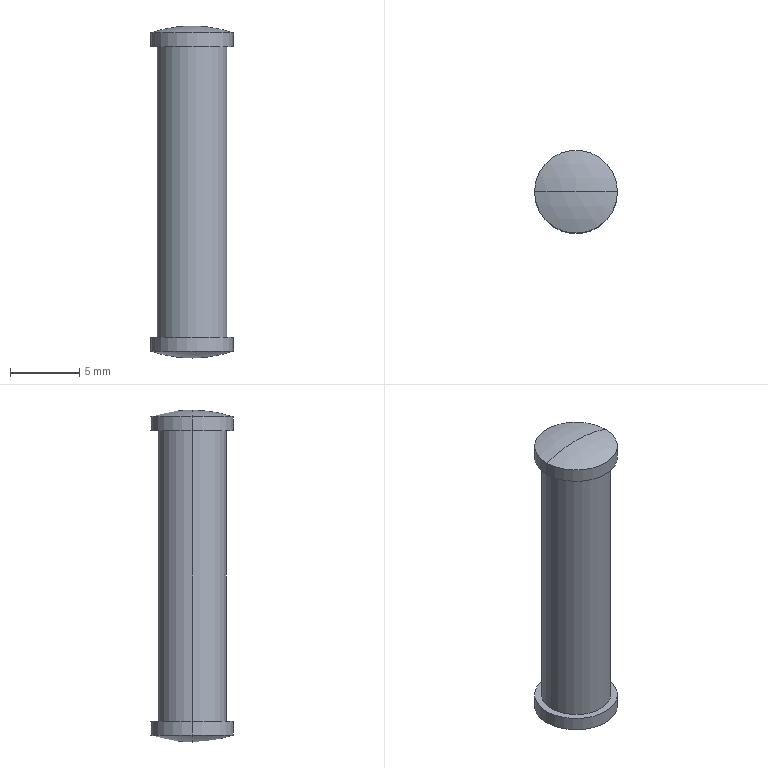Part | SolidWorks | features Dome 2, ICE 2, Extrusion 1 | 1 solid | 12 faces | box 6 x 6 x 24 mm | volume 483.151 mm3 | cylinder 6 | sphere 4 | plane 2 | commonest cylinder face diameters 6 x4 5 x2
STEP:
#1=CARTESIAN_POINT('',(3.,0.,11.5));
#2=VERTEX_POINT('',#1);
#3=CARTESIAN_POINT('',(-3.,0.,11.5));
#4=VERTEX_POINT('',#3);
#5=CARTESIAN_POINT('',(0.,0.,11.5));
#6=DIRECTION('',(0.,0.,1.));
#7=DIRECTION('',(1.,0.,0.));
#8=AXIS2_PLACEMENT_3D('',#5,#6,#7);
#9=CIRCLE('',#8,3.);
#10=EDGE_CURVE('',#2,#4,#9,.T.);
#11=ORIENTED_EDGE('',*,*,#10,.T.);
#12=CARTESIAN_POINT('',(0.,0.,12.));
#13=VERTEX_POINT('',#12);
#14=CARTESIAN_POINT('',(0.,0.,2.75));
#15=DIRECTION('',(0.,1.,0.));
#16=DIRECTION('',(-1.,0.,0.));
#17=AXIS2_PLACEMENT_3D('',#14,#15,#16);
#18=CIRCLE('',#17,9.25);
#19=EDGE_CURVE('',#4,#13,#18,.T.);
#20=ORIENTED_EDGE('',*,*,#19,.T.);
#21=CARTESIAN_POINT('',(0.,0.,2.75));
#22=DIRECTION('',(0.,-1.,0.));
#23=DIRECTION('',(0.,0.,-1.));
#24=AXIS2_PLACEMENT_3D('',#21,#22,#23);
#25=CIRCLE('',#24,9.25);
#26=EDGE_CURVE('',#2,#13,#25,.T.);
#27=ORIENTED_EDGE('',*,*,#26,.F.);
#28=EDGE_LOOP('',(#11,#20,#27));
#29=FACE_OUTER_BOUND('',#28,.T.);
#30=CARTESIAN_POINT('',(0.,0.,2.75));
#31=DIRECTION('',(0.,1.,0.));
#32=DIRECTION('',(1.,0.,0.));
#33=AXIS2_PLACEMENT_3D('',#30,#31,#32);
#34=SPHERICAL_SURFACE('',#33,9.25);
#35=ADVANCED_FACE('',(#29),#34,.T.);
#36=ORIENTED_EDGE('',*,*,#10,.F.);
#37=CARTESIAN_POINT('',(3.,0.,10.5));
#38=VERTEX_POINT('',#37);
#39=CARTESIAN_POINT('',(3.,0.,11.5));
#40=DIRECTION('',(0.,0.,-1.));
#41=VECTOR('',#40,1000.);
#42=LINE('',#39,#41);
#43=EDGE_CURVE('',#2,#38,#42,.T.);
#44=ORIENTED_EDGE('',*,*,#43,.T.);
#45=CARTESIAN_POINT('',(-3.,0.,10.5));
#46=VERTEX_POINT('',#45);
#47=CARTESIAN_POINT('',(0.,0.,10.5));
#48=DIRECTION('',(0.,0.,1.));
#49=DIRECTION('',(1.,0.,0.));
#50=AXIS2_PLACEMENT_3D('',#47,#48,#49);
#51=CIRCLE('',#50,3.);
#52=EDGE_CURVE('',#38,#46,#51,.T.);
#53=ORIENTED_EDGE('',*,*,#52,.T.);
#54=CARTESIAN_POINT('',(-3.,0.,11.5));
#55=DIRECTION('',(0.,0.,-1.));
#56=VECTOR('',#55,1000.);
#57=LINE('',#54,#56);
#58=EDGE_CURVE('',#4,#46,#57,.T.);
#59=ORIENTED_EDGE('',*,*,#58,.F.);
#60=EDGE_LOOP('',(#36,#44,#53,#59));
#61=FACE_OUTER_BOUND('',#60,.T.);
#62=CARTESIAN_POINT('',(0.,0.,11.5));
#63=DIRECTION('',(0.,0.,-1.));
#64=DIRECTION('',(-1.,0.,0.));
#65=AXIS2_PLACEMENT_3D('',#62,#63,#64);
#66=CYLINDRICAL_SURFACE('',#65,3.);
#67=ADVANCED_FACE('',(#61),#66,.T.);
#68=CARTESIAN_POINT('',(0.,0.,-12.));
#69=VERTEX_POINT('',#68);
#70=CARTESIAN_POINT('',(3.,0.,-11.5));
#71=VERTEX_POINT('',#70);
#72=CARTESIAN_POINT('',(0.,0.,-2.75));
#73=DIRECTION('',(0.,-1.,0.));
#74=DIRECTION('',(0.,0.,-1.));
#75=AXIS2_PLACEMENT_3D('',#72,#73,#74);
#76=CIRCLE('',#75,9.25);
#77=EDGE_CURVE('',#69,#71,#76,.T.);
#78=ORIENTED_EDGE('',*,*,#77,.F.);
#79=CARTESIAN_POINT('',(-3.,0.,-11.5));
#80=VERTEX_POINT('',#79);
#81=CARTESIAN_POINT('',(0.,0.,-2.75));
#82=DIRECTION('',(0.,1.,0.));
#83=DIRECTION('',(-1.,0.,0.));
#84=AXIS2_PLACEMENT_3D('',#81,#82,#83);
#85=CIRCLE('',#84,9.25);
#86=EDGE_CURVE('',#69,#80,#85,.T.);
#87=ORIENTED_EDGE('',*,*,#86,.T.);
#88=CARTESIAN_POINT('',(0.,0.,-11.5));
#89=DIRECTION('',(0.,0.,-1.));
#90=DIRECTION('',(-1.,0.,0.));
#91=AXIS2_PLACEMENT_3D('',#88,#89,#90);
#92=CIRCLE('',#91,3.);
#93=EDGE_CURVE('',#80,#71,#92,.T.);
#94=ORIENTED_EDGE('',*,*,#93,.T.);
#95=EDGE_LOOP('',(#78,#87,#94));
#96=FACE_OUTER_BOUND('',#95,.T.);
#97=CARTESIAN_POINT('',(0.,0.,-2.75));
#98=DIRECTION('',(0.,1.,0.));
#99=DIRECTION('',(1.,0.,0.));
#100=AXIS2_PLACEMENT_3D('',#97,#98,#99);
#101=SPHERICAL_SURFACE('',#100,9.25);
#102=ADVANCED_FACE('',(#96),#101,.T.);
#103=ORIENTED_EDGE('',*,*,#93,.F.);
#104=CARTESIAN_POINT('',(-3.,0.,-10.5));
#105=VERTEX_POINT('',#104);
#106=CARTESIAN_POINT('',(-3.,0.,-11.5));
#107=DIRECTION('',(0.,0.,1.));
#108=VECTOR('',#107,1000.);
#109=LINE('',#106,#108);
#110=EDGE_CURVE('',#80,#105,#109,.T.);
#111=ORIENTED_EDGE('',*,*,#110,.T.);
#112=CARTESIAN_POINT('',(3.,0.,-10.5));
#113=VERTEX_POINT('',#112);
#114=CARTESIAN_POINT('',(0.,0.,-10.5));
#115=DIRECTION('',(0.,0.,-1.));
#116=DIRECTION('',(-1.,0.,0.));
#117=AXIS2_PLACEMENT_3D('',#114,#115,#116);
#118=CIRCLE('',#117,3.);
#119=EDGE_CURVE('',#105,#113,#118,.T.);
#120=ORIENTED_EDGE('',*,*,#119,.T.);
#121=CARTESIAN_POINT('',(3.,0.,-11.5));
#122=DIRECTION('',(0.,0.,1.));
#123=VECTOR('',#122,1000.);
#124=LINE('',#121,#123);
#125=EDGE_CURVE('',#71,#113,#124,.T.);
#126=ORIENTED_EDGE('',*,*,#125,.F.);
#127=EDGE_LOOP('',(#103,#111,#120,#126));
#128=FACE_OUTER_BOUND('',#127,.T.);
#129=CARTESIAN_POINT('',(0.,0.,-11.5));
#130=DIRECTION('',(0.,0.,1.));
#131=DIRECTION('',(1.,0.,0.));
#132=AXIS2_PLACEMENT_3D('',#129,#130,#131);
#133=CYLINDRICAL_SURFACE('',#132,3.);
#134=ADVANCED_FACE('',(#128),#133,.T.);
#135=CARTESIAN_POINT('',(2.5,0.,10.5));
#136=VERTEX_POINT('',#135);
#137=CARTESIAN_POINT('',(-2.5,0.,10.5));
#138=VERTEX_POINT('',#137);
#139=CARTESIAN_POINT('',(0.,0.,10.5));
#140=DIRECTION('',(0.,0.,1.));
#141=DIRECTION('',(1.,0.,0.));
#142=AXIS2_PLACEMENT_3D('',#139,#140,#141);
#143=CIRCLE('',#142,2.5);
#144=EDGE_CURVE('',#136,#138,#143,.T.);
#145=ORIENTED_EDGE('',*,*,#144,.F.);
#146=CARTESIAN_POINT('',(2.5,0.,-10.5));
#147=VERTEX_POINT('',#146);
#148=CARTESIAN_POINT('',(2.5,0.,10.5));
#149=DIRECTION('',(0.,0.,-1.));
#150=VECTOR('',#149,1000.);
#151=LINE('',#148,#150);
#152=EDGE_CURVE('',#136,#147,#151,.T.);
#153=ORIENTED_EDGE('',*,*,#152,.T.);
#154=CARTESIAN_POINT('',(-2.5,0.,-10.5));
#155=VERTEX_POINT('',#154);
#156=CARTESIAN_POINT('',(0.,0.,-10.5));
#157=DIRECTION('',(0.,0.,-1.));
#158=DIRECTION('',(-1.,0.,0.));
#159=AXIS2_PLACEMENT_3D('',#156,#157,#158);
#160=CIRCLE('',#159,2.5);
#161=EDGE_CURVE('',#155,#147,#160,.T.);
#162=ORIENTED_EDGE('',*,*,#161,.F.);
#163=CARTESIAN_POINT('',(-2.5,0.,10.5));
#164=DIRECTION('',(0.,0.,-1.));
#165=VECTOR('',#164,1000.);
#166=LINE('',#163,#165);
#167=EDGE_CURVE('',#138,#155,#166,.T.);
#168=ORIENTED_EDGE('',*,*,#167,.F.);
#169=EDGE_LOOP('',(#145,#153,#162,#168));
#170=FACE_OUTER_BOUND('',#169,.T.);
#171=CARTESIAN_POINT('',(0.,0.,10.5));
#172=DIRECTION('',(0.,0.,-1.));
#173=DIRECTION('',(-1.,0.,0.));
#174=AXIS2_PLACEMENT_3D('',#171,#172,#173);
#175=CYLINDRICAL_SURFACE('',#174,2.5);
#176=ADVANCED_FACE('',(#170),#175,.T.);
#177=ORIENTED_EDGE('',*,*,#152,.F.);
#178=CARTESIAN_POINT('',(0.,0.,10.5));
#179=DIRECTION('',(0.,0.,1.));
#180=DIRECTION('',(1.,0.,0.));
#181=AXIS2_PLACEMENT_3D('',#178,#179,#180);
#182=CIRCLE('',#181,2.5);
#183=EDGE_CURVE('',#138,#136,#182,.T.);
#184=ORIENTED_EDGE('',*,*,#183,.F.);
#185=ORIENTED_EDGE('',*,*,#167,.T.);
#186=CARTESIAN_POINT('',(0.,0.,-10.5));
#187=DIRECTION('',(0.,0.,-1.));
#188=DIRECTION('',(-1.,0.,0.));
#189=AXIS2_PLACEMENT_3D('',#186,#187,#188);
#190=CIRCLE('',#189,2.5);
#191=EDGE_CURVE('',#147,#155,#190,.T.);
#192=ORIENTED_EDGE('',*,*,#191,.F.);
#193=EDGE_LOOP('',(#177,#184,#185,#192));
#194=FACE_OUTER_BOUND('',#193,.T.);
#195=CARTESIAN_POINT('',(0.,0.,10.5));
#196=DIRECTION('',(0.,0.,-1.));
#197=DIRECTION('',(-1.,0.,0.));
#198=AXIS2_PLACEMENT_3D('',#195,#196,#197);
#199=CYLINDRICAL_SURFACE('',#198,2.5);
#200=ADVANCED_FACE('',(#194),#199,.T.);
#201=CARTESIAN_POINT('',(0.,0.,-10.5));
#202=DIRECTION('',(0.,0.,-1.));
#203=DIRECTION('',(-1.,0.,0.));
#204=AXIS2_PLACEMENT_3D('',#201,#202,#203);
#205=CIRCLE('',#204,3.);
#206=EDGE_CURVE('',#113,#105,#205,.T.);
#207=ORIENTED_EDGE('',*,*,#206,.F.);
#208=ORIENTED_EDGE('',*,*,#119,.F.);
#209=EDGE_LOOP('',(#207,#208));
#210=FACE_OUTER_BOUND('',#209,.T.);
#211=ORIENTED_EDGE('',*,*,#161,.T.);
#212=ORIENTED_EDGE('',*,*,#191,.T.);
#213=EDGE_LOOP('',(#211,#212));
#214=FACE_BOUND('',#213,.T.);
#215=CARTESIAN_POINT('',(0.,0.,-10.5));
#216=DIRECTION('',(0.,0.,-1.));
#217=DIRECTION('',(-1.,0.,0.));
#218=AXIS2_PLACEMENT_3D('',#215,#216,#217);
#219=PLANE('',#218);
#220=ADVANCED_FACE('',(#210,#214),#219,.F.);
#221=ORIENTED_EDGE('',*,*,#110,.F.);
#222=CARTESIAN_POINT('',(0.,0.,-11.5));
#223=DIRECTION('',(0.,0.,-1.));
#224=DIRECTION('',(-1.,0.,0.));
#225=AXIS2_PLACEMENT_3D('',#222,#223,#224);
#226=CIRCLE('',#225,3.);
#227=EDGE_CURVE('',#71,#80,#226,.T.);
#228=ORIENTED_EDGE('',*,*,#227,.F.);
#229=ORIENTED_EDGE('',*,*,#125,.T.);
#230=ORIENTED_EDGE('',*,*,#206,.T.);
#231=EDGE_LOOP('',(#221,#228,#229,#230));
#232=FACE_OUTER_BOUND('',#231,.T.);
#233=CARTESIAN_POINT('',(0.,0.,-11.5));
#234=DIRECTION('',(0.,0.,1.));
#235=DIRECTION('',(1.,0.,0.));
#236=AXIS2_PLACEMENT_3D('',#233,#234,#235);
#237=CYLINDRICAL_SURFACE('',#236,3.);
#238=ADVANCED_FACE('',(#232),#237,.T.);
#239=ORIENTED_EDGE('',*,*,#86,.F.);
#240=ORIENTED_EDGE('',*,*,#77,.T.);
#241=ORIENTED_EDGE('',*,*,#227,.T.);
#242=EDGE_LOOP('',(#239,#240,#241));
#243=FACE_OUTER_BOUND('',#242,.T.);
#244=CARTESIAN_POINT('',(0.,0.,-2.75));
#245=DIRECTION('',(0.,1.,0.));
#246=DIRECTION('',(1.,0.,0.));
#247=AXIS2_PLACEMENT_3D('',#244,#245,#246);
#248=SPHERICAL_SURFACE('',#247,9.25);
#249=ADVANCED_FACE('',(#243),#248,.T.);
#250=CARTESIAN_POINT('',(0.,0.,10.5));
#251=DIRECTION('',(0.,0.,1.));
#252=DIRECTION('',(1.,0.,0.));
#253=AXIS2_PLACEMENT_3D('',#250,#251,#252);
#254=CIRCLE('',#253,3.);
#255=EDGE_CURVE('',#46,#38,#254,.T.);
#256=ORIENTED_EDGE('',*,*,#255,.F.);
#257=ORIENTED_EDGE('',*,*,#52,.F.);
#258=EDGE_LOOP('',(#256,#257));
#259=FACE_OUTER_BOUND('',#258,.T.);
#260=ORIENTED_EDGE('',*,*,#183,.T.);
#261=ORIENTED_EDGE('',*,*,#144,.T.);
#262=EDGE_LOOP('',(#260,#261));
#263=FACE_BOUND('',#262,.T.);
#264=CARTESIAN_POINT('',(0.,0.,10.5));
#265=DIRECTION('',(0.,0.,1.));
#266=DIRECTION('',(1.,0.,0.));
#267=AXIS2_PLACEMENT_3D('',#264,#265,#266);
#268=PLANE('',#267);
#269=ADVANCED_FACE('',(#259,#263),#268,.F.);
#270=ORIENTED_EDGE('',*,*,#43,.F.);
#271=CARTESIAN_POINT('',(0.,0.,11.5));
#272=DIRECTION('',(0.,0.,1.));
#273=DIRECTION('',(1.,0.,0.));
#274=AXIS2_PLACEMENT_3D('',#271,#272,#273);
#275=CIRCLE('',#274,3.);
#276=EDGE_CURVE('',#4,#2,#275,.T.);
#277=ORIENTED_EDGE('',*,*,#276,.F.);
#278=ORIENTED_EDGE('',*,*,#58,.T.);
#279=ORIENTED_EDGE('',*,*,#255,.T.);
#280=EDGE_LOOP('',(#270,#277,#278,#279));
#281=FACE_OUTER_BOUND('',#280,.T.);
#282=CARTESIAN_POINT('',(0.,0.,11.5));
#283=DIRECTION('',(0.,0.,-1.));
#284=DIRECTION('',(-1.,0.,0.));
#285=AXIS2_PLACEMENT_3D('',#282,#283,#284);
#286=CYLINDRICAL_SURFACE('',#285,3.);
#287=ADVANCED_FACE('',(#281),#286,.T.);
#288=ORIENTED_EDGE('',*,*,#19,.F.);
#289=ORIENTED_EDGE('',*,*,#276,.T.);
#290=ORIENTED_EDGE('',*,*,#26,.T.);
#291=EDGE_LOOP('',(#288,#289,#290));
#292=FACE_OUTER_BOUND('',#291,.T.);
#293=CARTESIAN_POINT('',(0.,0.,2.75));
#294=DIRECTION('',(0.,1.,0.));
#295=DIRECTION('',(1.,0.,0.));
#296=AXIS2_PLACEMENT_3D('',#293,#294,#295);
#297=SPHERICAL_SURFACE('',#296,9.25);
#298=ADVANCED_FACE('',(#292),#297,.T.);
#299=CLOSED_SHELL('',(#35,#67,#102,#134,#176,#200,#220,#238,#249,#269,#287,#298));
#300=MANIFOLD_SOLID_BREP('',#299);
#301=CARTESIAN_POINT('',(0.,0.,0.));
#302=DIRECTION('',(0.,0.,1.));
#303=DIRECTION('',(1.,0.,0.));
#304=AXIS2_PLACEMENT_3D('',#301,#302,#303);
#305=(LENGTH_UNIT()NAMED_UNIT(*)SI_UNIT(.MILLI.,.METRE.));
#306=UNCERTAINTY_MEASURE_WITH_UNIT(LENGTH_MEASURE(0.00001),#305,'','');
#307=(NAMED_UNIT(*)PLANE_ANGLE_UNIT()SI_UNIT($,.RADIAN.));
#308=(NAMED_UNIT(*)SI_UNIT($,.STERADIAN.)SOLID_ANGLE_UNIT());
#309=(GEOMETRIC_REPRESENTATION_CONTEXT(3)GLOBAL_UNCERTAINTY_ASSIGNED_CONTEXT((#306))GLOBAL_UNIT_ASSIGNED_CONTEXT((#305,#307,#308))REPRESENTATION_CONTEXT('',''));
#310=ADVANCED_BREP_SHAPE_REPRESENTATION('',(#300,#304),#309);